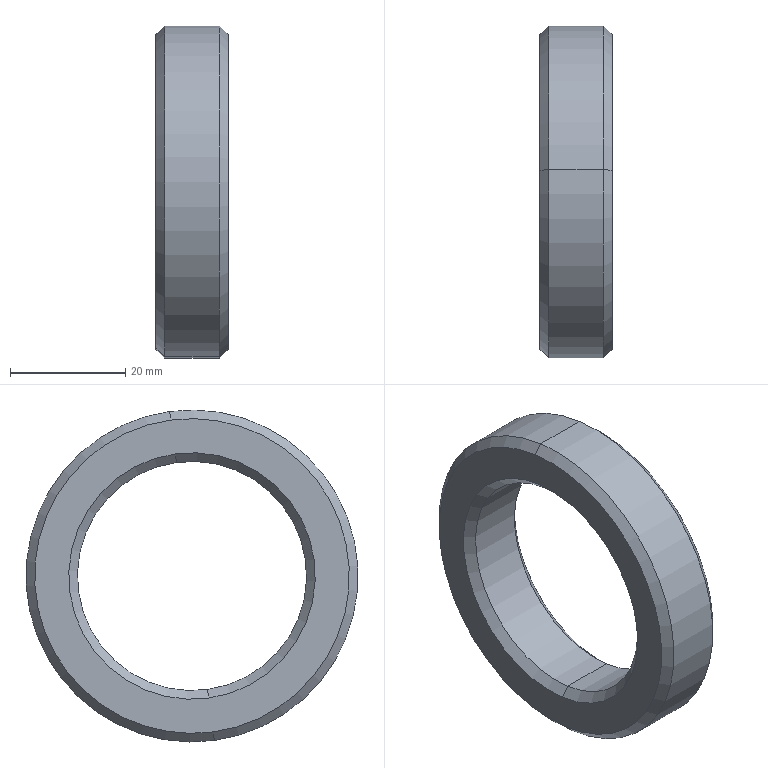Part | NX | features BREP 1 | 1 solid | 14 faces | box 12.5 x 57.5 x 57.5 mm | volume 16308 mm3 | cone 8 | cylinder 4 | plane 2 | commonest cylinder face diameters 39.688 x2 57.5 x2
STEP:
#1=CARTESIAN_POINT('',(-576.92,3.677,27.001));
#2=VERTEX_POINT('',#1);
#3=CARTESIAN_POINT('',(-576.92,-3.677,-27.001));
#4=VERTEX_POINT('',#3);
#5=CARTESIAN_POINT('',(-576.92,0.,0.));
#6=DIRECTION('',(-1.,0.,0.));
#7=DIRECTION('',(0.,0.1349,0.9909));
#8=AXIS2_PLACEMENT_3D('',#5,#6,#7);
#9=CIRCLE('',#8,27.25);
#10=EDGE_CURVE('',#2,#4,#9,.T.);
#11=ORIENTED_EDGE('',*,*,#10,.T.);
#12=CARTESIAN_POINT('',(-578.42,-3.879,-28.487));
#13=VERTEX_POINT('',#12);
#14=CARTESIAN_POINT('',(-576.92,-3.677,-27.001));
#15=DIRECTION('',(-0.7071,-0.09541,-0.7006));
#16=VECTOR('',#15,1000.);
#17=LINE('',#14,#16);
#18=EDGE_CURVE('',#4,#13,#17,.T.);
#19=ORIENTED_EDGE('',*,*,#18,.T.);
#20=CARTESIAN_POINT('',(-578.42,3.879,28.487));
#21=VERTEX_POINT('',#20);
#22=CARTESIAN_POINT('',(-578.42,0.,0.));
#23=DIRECTION('',(-1.,0.,0.));
#24=DIRECTION('',(0.,0.1349,0.9909));
#25=AXIS2_PLACEMENT_3D('',#22,#23,#24);
#26=CIRCLE('',#25,28.75);
#27=EDGE_CURVE('',#21,#13,#26,.T.);
#28=ORIENTED_EDGE('',*,*,#27,.F.);
#29=CARTESIAN_POINT('',(-576.92,3.677,27.001));
#30=DIRECTION('',(-0.7071,0.09541,0.7006));
#31=VECTOR('',#30,1000.);
#32=LINE('',#29,#31);
#33=EDGE_CURVE('',#2,#21,#32,.T.);
#34=ORIENTED_EDGE('',*,*,#33,.F.);
#35=EDGE_LOOP('',(#11,#19,#28,#34));
#36=FACE_BOUND('',#35,.T.);
#37=CARTESIAN_POINT('',(-576.92,0.,0.));
#38=DIRECTION('',(-1.,0.,0.));
#39=DIRECTION('',(0.,-0.1349,-0.9909));
#40=AXIS2_PLACEMENT_3D('',#37,#38,#39);
#41=CONICAL_SURFACE('',#40,27.25,0.7854);
#42=ADVANCED_FACE('',(#36),#41,.T.);
#43=CARTESIAN_POINT('',(-578.42,-2.678,-19.663));
#44=VERTEX_POINT('',#43);
#45=CARTESIAN_POINT('',(-578.42,2.678,19.663));
#46=VERTEX_POINT('',#45);
#47=CARTESIAN_POINT('',(-578.42,0.,0.));
#48=DIRECTION('',(-1.,0.,0.));
#49=DIRECTION('',(0.,0.1349,0.9909));
#50=AXIS2_PLACEMENT_3D('',#47,#48,#49);
#51=CIRCLE('',#50,19.844);
#52=EDGE_CURVE('',#44,#46,#51,.T.);
#53=ORIENTED_EDGE('',*,*,#52,.T.);
#54=CARTESIAN_POINT('',(-576.92,2.88,21.149));
#55=VERTEX_POINT('',#54);
#56=CARTESIAN_POINT('',(-578.42,2.678,19.663));
#57=DIRECTION('',(0.7071,0.09541,0.7006));
#58=VECTOR('',#57,1000.);
#59=LINE('',#56,#58);
#60=EDGE_CURVE('',#55,#46,#59,.F.);
#61=ORIENTED_EDGE('',*,*,#60,.F.);
#62=CARTESIAN_POINT('',(-576.92,-2.88,-21.149));
#63=VERTEX_POINT('',#62);
#64=CARTESIAN_POINT('',(-576.92,0.,0.));
#65=DIRECTION('',(-1.,0.,0.));
#66=DIRECTION('',(0.,0.1349,0.9909));
#67=AXIS2_PLACEMENT_3D('',#64,#65,#66);
#68=CIRCLE('',#67,21.344);
#69=EDGE_CURVE('',#63,#55,#68,.T.);
#70=ORIENTED_EDGE('',*,*,#69,.F.);
#71=CARTESIAN_POINT('',(-578.42,-2.678,-19.663));
#72=DIRECTION('',(0.7071,-0.09541,-0.7006));
#73=VECTOR('',#72,1000.);
#74=LINE('',#71,#73);
#75=EDGE_CURVE('',#63,#44,#74,.F.);
#76=ORIENTED_EDGE('',*,*,#75,.T.);
#77=EDGE_LOOP('',(#53,#61,#70,#76));
#78=FACE_BOUND('',#77,.T.);
#79=CARTESIAN_POINT('',(-578.42,0.,0.));
#80=DIRECTION('',(1.,0.,0.));
#81=DIRECTION('',(0.,0.1349,0.9909));
#82=AXIS2_PLACEMENT_3D('',#79,#80,#81);
#83=CONICAL_SURFACE('',#82,19.844,0.7854);
#84=ADVANCED_FACE('',(#78),#83,.F.);
#85=ORIENTED_EDGE('',*,*,#52,.F.);
#86=CARTESIAN_POINT('',(-587.92,-2.678,-19.663));
#87=VERTEX_POINT('',#86);
#88=CARTESIAN_POINT('',(-589.42,-2.678,-19.663));
#89=DIRECTION('',(-1.,0.,0.));
#90=VECTOR('',#89,1000.);
#91=LINE('',#88,#90);
#92=EDGE_CURVE('',#44,#87,#91,.T.);
#93=ORIENTED_EDGE('',*,*,#92,.T.);
#94=CARTESIAN_POINT('',(-587.92,2.678,19.663));
#95=VERTEX_POINT('',#94);
#96=CARTESIAN_POINT('',(-587.92,0.,0.));
#97=DIRECTION('',(-1.,0.,0.));
#98=DIRECTION('',(0.,0.1349,0.9909));
#99=AXIS2_PLACEMENT_3D('',#96,#97,#98);
#100=CIRCLE('',#99,19.844);
#101=EDGE_CURVE('',#87,#95,#100,.T.);
#102=ORIENTED_EDGE('',*,*,#101,.T.);
#103=CARTESIAN_POINT('',(-589.42,2.678,19.663));
#104=DIRECTION('',(-1.,0.,0.));
#105=VECTOR('',#104,1000.);
#106=LINE('',#103,#105);
#107=EDGE_CURVE('',#46,#95,#106,.T.);
#108=ORIENTED_EDGE('',*,*,#107,.F.);
#109=EDGE_LOOP('',(#85,#93,#102,#108));
#110=FACE_BOUND('',#109,.T.);
#111=CARTESIAN_POINT('',(-589.42,0.,0.));
#112=DIRECTION('',(-1.,0.,0.));
#113=DIRECTION('',(0.,-0.1349,-0.9909));
#114=AXIS2_PLACEMENT_3D('',#111,#112,#113);
#115=CYLINDRICAL_SURFACE('',#114,19.844);
#116=ADVANCED_FACE('',(#110),#115,.F.);
#117=ORIENTED_EDGE('',*,*,#101,.F.);
#118=CARTESIAN_POINT('',(-589.42,-2.88,-21.149));
#119=VERTEX_POINT('',#118);
#120=CARTESIAN_POINT('',(-589.42,-2.88,-21.149));
#121=DIRECTION('',(-0.7071,-0.09541,-0.7006));
#122=VECTOR('',#121,1000.);
#123=LINE('',#120,#122);
#124=EDGE_CURVE('',#87,#119,#123,.T.);
#125=ORIENTED_EDGE('',*,*,#124,.T.);
#126=CARTESIAN_POINT('',(-589.42,2.88,21.149));
#127=VERTEX_POINT('',#126);
#128=CARTESIAN_POINT('',(-589.42,0.,0.));
#129=DIRECTION('',(-1.,0.,0.));
#130=DIRECTION('',(0.,0.1349,0.9909));
#131=AXIS2_PLACEMENT_3D('',#128,#129,#130);
#132=CIRCLE('',#131,21.344);
#133=EDGE_CURVE('',#119,#127,#132,.T.);
#134=ORIENTED_EDGE('',*,*,#133,.T.);
#135=CARTESIAN_POINT('',(-589.42,2.88,21.149));
#136=DIRECTION('',(-0.7071,0.09541,0.7006));
#137=VECTOR('',#136,1000.);
#138=LINE('',#135,#137);
#139=EDGE_CURVE('',#95,#127,#138,.T.);
#140=ORIENTED_EDGE('',*,*,#139,.F.);
#141=EDGE_LOOP('',(#117,#125,#134,#140));
#142=FACE_BOUND('',#141,.T.);
#143=CARTESIAN_POINT('',(-589.42,0.,0.));
#144=DIRECTION('',(-1.,0.,0.));
#145=DIRECTION('',(0.,-0.1349,-0.9909));
#146=AXIS2_PLACEMENT_3D('',#143,#144,#145);
#147=CONICAL_SURFACE('',#146,21.344,0.7854);
#148=ADVANCED_FACE('',(#142),#147,.F.);
#149=CARTESIAN_POINT('',(-589.42,3.677,27.001));
#150=VERTEX_POINT('',#149);
#151=CARTESIAN_POINT('',(-589.42,-3.677,-27.001));
#152=VERTEX_POINT('',#151);
#153=CARTESIAN_POINT('',(-589.42,0.,0.));
#154=DIRECTION('',(-1.,0.,0.));
#155=DIRECTION('',(0.,0.1349,0.9909));
#156=AXIS2_PLACEMENT_3D('',#153,#154,#155);
#157=CIRCLE('',#156,27.25);
#158=EDGE_CURVE('',#150,#152,#157,.T.);
#159=ORIENTED_EDGE('',*,*,#158,.F.);
#160=CARTESIAN_POINT('',(-587.92,3.879,28.487));
#161=VERTEX_POINT('',#160);
#162=CARTESIAN_POINT('',(-587.92,3.879,28.487));
#163=DIRECTION('',(0.7071,0.09541,0.7006));
#164=VECTOR('',#163,1000.);
#165=LINE('',#162,#164);
#166=EDGE_CURVE('',#161,#150,#165,.F.);
#167=ORIENTED_EDGE('',*,*,#166,.F.);
#168=CARTESIAN_POINT('',(-587.92,-3.879,-28.487));
#169=VERTEX_POINT('',#168);
#170=CARTESIAN_POINT('',(-587.92,0.,0.));
#171=DIRECTION('',(-1.,0.,0.));
#172=DIRECTION('',(0.,0.1349,0.9909));
#173=AXIS2_PLACEMENT_3D('',#170,#171,#172);
#174=CIRCLE('',#173,28.75);
#175=EDGE_CURVE('',#161,#169,#174,.T.);
#176=ORIENTED_EDGE('',*,*,#175,.T.);
#177=CARTESIAN_POINT('',(-587.92,-3.879,-28.487));
#178=DIRECTION('',(0.7071,-0.09541,-0.7006));
#179=VECTOR('',#178,1000.);
#180=LINE('',#177,#179);
#181=EDGE_CURVE('',#169,#152,#180,.F.);
#182=ORIENTED_EDGE('',*,*,#181,.T.);
#183=EDGE_LOOP('',(#159,#167,#176,#182));
#184=FACE_BOUND('',#183,.T.);
#185=CARTESIAN_POINT('',(-587.92,0.,0.));
#186=DIRECTION('',(1.,0.,0.));
#187=DIRECTION('',(0.,0.1349,0.9909));
#188=AXIS2_PLACEMENT_3D('',#185,#186,#187);
#189=CONICAL_SURFACE('',#188,28.75,0.7854);
#190=ADVANCED_FACE('',(#184),#189,.T.);
#191=ORIENTED_EDGE('',*,*,#27,.T.);
#192=CARTESIAN_POINT('',(-589.42,-3.879,-28.487));
#193=DIRECTION('',(-1.,0.,0.));
#194=VECTOR('',#193,1000.);
#195=LINE('',#192,#194);
#196=EDGE_CURVE('',#13,#169,#195,.T.);
#197=ORIENTED_EDGE('',*,*,#196,.T.);
#198=ORIENTED_EDGE('',*,*,#175,.F.);
#199=CARTESIAN_POINT('',(-589.42,3.879,28.487));
#200=DIRECTION('',(-1.,0.,0.));
#201=VECTOR('',#200,1000.);
#202=LINE('',#199,#201);
#203=EDGE_CURVE('',#21,#161,#202,.T.);
#204=ORIENTED_EDGE('',*,*,#203,.F.);
#205=EDGE_LOOP('',(#191,#197,#198,#204));
#206=FACE_BOUND('',#205,.T.);
#207=CARTESIAN_POINT('',(-589.42,0.,0.));
#208=DIRECTION('',(-1.,0.,0.));
#209=DIRECTION('',(0.,-0.1349,-0.9909));
#210=AXIS2_PLACEMENT_3D('',#207,#208,#209);
#211=CYLINDRICAL_SURFACE('',#210,28.75);
#212=ADVANCED_FACE('',(#206),#211,.T.);
#213=ORIENTED_EDGE('',*,*,#196,.F.);
#214=CARTESIAN_POINT('',(-578.42,0.,0.));
#215=DIRECTION('',(-1.,0.,0.));
#216=DIRECTION('',(0.,0.1349,0.9909));
#217=AXIS2_PLACEMENT_3D('',#214,#215,#216);
#218=CIRCLE('',#217,28.75);
#219=EDGE_CURVE('',#13,#21,#218,.T.);
#220=ORIENTED_EDGE('',*,*,#219,.T.);
#221=ORIENTED_EDGE('',*,*,#203,.T.);
#222=CARTESIAN_POINT('',(-587.92,0.,0.));
#223=DIRECTION('',(-1.,0.,0.));
#224=DIRECTION('',(0.,0.1349,0.9909));
#225=AXIS2_PLACEMENT_3D('',#222,#223,#224);
#226=CIRCLE('',#225,28.75);
#227=EDGE_CURVE('',#169,#161,#226,.T.);
#228=ORIENTED_EDGE('',*,*,#227,.F.);
#229=EDGE_LOOP('',(#213,#220,#221,#228));
#230=FACE_BOUND('',#229,.T.);
#231=CARTESIAN_POINT('',(-589.42,0.,0.));
#232=DIRECTION('',(-1.,0.,0.));
#233=DIRECTION('',(0.,-0.1349,-0.9909));
#234=AXIS2_PLACEMENT_3D('',#231,#232,#233);
#235=CYLINDRICAL_SURFACE('',#234,28.75);
#236=ADVANCED_FACE('',(#230),#235,.T.);
#237=ORIENTED_EDGE('',*,*,#166,.T.);
#238=CARTESIAN_POINT('',(-589.42,0.,0.));
#239=DIRECTION('',(-1.,0.,0.));
#240=DIRECTION('',(0.,0.1349,0.9909));
#241=AXIS2_PLACEMENT_3D('',#238,#239,#240);
#242=CIRCLE('',#241,27.25);
#243=EDGE_CURVE('',#152,#150,#242,.T.);
#244=ORIENTED_EDGE('',*,*,#243,.F.);
#245=ORIENTED_EDGE('',*,*,#181,.F.);
#246=ORIENTED_EDGE('',*,*,#227,.T.);
#247=EDGE_LOOP('',(#237,#244,#245,#246));
#248=FACE_BOUND('',#247,.T.);
#249=CARTESIAN_POINT('',(-587.92,0.,0.));
#250=DIRECTION('',(1.,0.,0.));
#251=DIRECTION('',(0.,0.1349,0.9909));
#252=AXIS2_PLACEMENT_3D('',#249,#250,#251);
#253=CONICAL_SURFACE('',#252,28.75,0.7854);
#254=ADVANCED_FACE('',(#248),#253,.T.);
#255=CARTESIAN_POINT('',(-589.42,0.,0.));
#256=DIRECTION('',(-1.,0.,0.));
#257=DIRECTION('',(0.,0.1349,0.9909));
#258=AXIS2_PLACEMENT_3D('',#255,#256,#257);
#259=CIRCLE('',#258,21.344);
#260=EDGE_CURVE('',#127,#119,#259,.T.);
#261=ORIENTED_EDGE('',*,*,#260,.F.);
#262=ORIENTED_EDGE('',*,*,#133,.F.);
#263=EDGE_LOOP('',(#261,#262));
#264=FACE_BOUND('',#263,.T.);
#265=ORIENTED_EDGE('',*,*,#243,.T.);
#266=ORIENTED_EDGE('',*,*,#158,.T.);
#267=EDGE_LOOP('',(#265,#266));
#268=FACE_BOUND('',#267,.T.);
#269=CARTESIAN_POINT('',(-589.42,27.001,-3.677));
#270=DIRECTION('',(1.,0.,0.));
#271=DIRECTION('',(0.,0.1349,0.9909));
#272=AXIS2_PLACEMENT_3D('',#269,#270,#271);
#273=PLANE('',#272);
#274=ADVANCED_FACE('',(#264,#268),#273,.F.);
#275=ORIENTED_EDGE('',*,*,#124,.F.);
#276=CARTESIAN_POINT('',(-587.92,0.,0.));
#277=DIRECTION('',(-1.,0.,0.));
#278=DIRECTION('',(0.,0.1349,0.9909));
#279=AXIS2_PLACEMENT_3D('',#276,#277,#278);
#280=CIRCLE('',#279,19.844);
#281=EDGE_CURVE('',#95,#87,#280,.T.);
#282=ORIENTED_EDGE('',*,*,#281,.F.);
#283=ORIENTED_EDGE('',*,*,#139,.T.);
#284=ORIENTED_EDGE('',*,*,#260,.T.);
#285=EDGE_LOOP('',(#275,#282,#283,#284));
#286=FACE_BOUND('',#285,.T.);
#287=CARTESIAN_POINT('',(-589.42,0.,0.));
#288=DIRECTION('',(-1.,0.,0.));
#289=DIRECTION('',(0.,-0.1349,-0.9909));
#290=AXIS2_PLACEMENT_3D('',#287,#288,#289);
#291=CONICAL_SURFACE('',#290,21.344,0.7854);
#292=ADVANCED_FACE('',(#286),#291,.F.);
#293=ORIENTED_EDGE('',*,*,#92,.F.);
#294=CARTESIAN_POINT('',(-578.42,0.,0.));
#295=DIRECTION('',(-1.,0.,0.));
#296=DIRECTION('',(0.,0.1349,0.9909));
#297=AXIS2_PLACEMENT_3D('',#294,#295,#296);
#298=CIRCLE('',#297,19.844);
#299=EDGE_CURVE('',#46,#44,#298,.T.);
#300=ORIENTED_EDGE('',*,*,#299,.F.);
#301=ORIENTED_EDGE('',*,*,#107,.T.);
#302=ORIENTED_EDGE('',*,*,#281,.T.);
#303=EDGE_LOOP('',(#293,#300,#301,#302));
#304=FACE_BOUND('',#303,.T.);
#305=CARTESIAN_POINT('',(-589.42,0.,0.));
#306=DIRECTION('',(-1.,0.,0.));
#307=DIRECTION('',(0.,-0.1349,-0.9909));
#308=AXIS2_PLACEMENT_3D('',#305,#306,#307);
#309=CYLINDRICAL_SURFACE('',#308,19.844);
#310=ADVANCED_FACE('',(#304),#309,.F.);
#311=ORIENTED_EDGE('',*,*,#60,.T.);
#312=ORIENTED_EDGE('',*,*,#299,.T.);
#313=ORIENTED_EDGE('',*,*,#75,.F.);
#314=CARTESIAN_POINT('',(-576.92,0.,0.));
#315=DIRECTION('',(-1.,0.,0.));
#316=DIRECTION('',(0.,0.1349,0.9909));
#317=AXIS2_PLACEMENT_3D('',#314,#315,#316);
#318=CIRCLE('',#317,21.344);
#319=EDGE_CURVE('',#55,#63,#318,.T.);
#320=ORIENTED_EDGE('',*,*,#319,.F.);
#321=EDGE_LOOP('',(#311,#312,#313,#320));
#322=FACE_BOUND('',#321,.T.);
#323=CARTESIAN_POINT('',(-578.42,0.,0.));
#324=DIRECTION('',(1.,0.,0.));
#325=DIRECTION('',(0.,0.1349,0.9909));
#326=AXIS2_PLACEMENT_3D('',#323,#324,#325);
#327=CONICAL_SURFACE('',#326,19.844,0.7854);
#328=ADVANCED_FACE('',(#322),#327,.F.);
#329=ORIENTED_EDGE('',*,*,#10,.F.);
#330=CARTESIAN_POINT('',(-576.92,0.,0.));
#331=DIRECTION('',(-1.,0.,0.));
#332=DIRECTION('',(0.,0.1349,0.9909));
#333=AXIS2_PLACEMENT_3D('',#330,#331,#332);
#334=CIRCLE('',#333,27.25);
#335=EDGE_CURVE('',#4,#2,#334,.T.);
#336=ORIENTED_EDGE('',*,*,#335,.F.);
#337=EDGE_LOOP('',(#329,#336));
#338=FACE_BOUND('',#337,.T.);
#339=ORIENTED_EDGE('',*,*,#69,.T.);
#340=ORIENTED_EDGE('',*,*,#319,.T.);
#341=EDGE_LOOP('',(#339,#340));
#342=FACE_BOUND('',#341,.T.);
#343=CARTESIAN_POINT('',(-576.92,21.149,-2.88));
#344=DIRECTION('',(-1.,0.,0.));
#345=DIRECTION('',(0.,-0.1349,-0.9909));
#346=AXIS2_PLACEMENT_3D('',#343,#344,#345);
#347=PLANE('',#346);
#348=ADVANCED_FACE('',(#338,#342),#347,.F.);
#349=ORIENTED_EDGE('',*,*,#18,.F.);
#350=ORIENTED_EDGE('',*,*,#335,.T.);
#351=ORIENTED_EDGE('',*,*,#33,.T.);
#352=ORIENTED_EDGE('',*,*,#219,.F.);
#353=EDGE_LOOP('',(#349,#350,#351,#352));
#354=FACE_BOUND('',#353,.T.);
#355=CARTESIAN_POINT('',(-576.92,0.,0.));
#356=DIRECTION('',(-1.,0.,0.));
#357=DIRECTION('',(0.,-0.1349,-0.9909));
#358=AXIS2_PLACEMENT_3D('',#355,#356,#357);
#359=CONICAL_SURFACE('',#358,27.25,0.7854);
#360=ADVANCED_FACE('',(#354),#359,.T.);
#361=CLOSED_SHELL('',(#42,#84,#116,#148,#190,#212,#236,#254,#274,#292,#310,#328,#348,#360));
#362=MANIFOLD_SOLID_BREP('',#361);
#363=(LENGTH_UNIT()NAMED_UNIT(*)SI_UNIT(.MILLI.,.METRE.));
#364=UNCERTAINTY_MEASURE_WITH_UNIT(LENGTH_MEASURE(0.00001),#363,'','');
#365=(NAMED_UNIT(*)PLANE_ANGLE_UNIT()SI_UNIT($,.RADIAN.));
#366=(NAMED_UNIT(*)SI_UNIT($,.STERADIAN.)SOLID_ANGLE_UNIT());
#367=(GEOMETRIC_REPRESENTATION_CONTEXT(3)GLOBAL_UNCERTAINTY_ASSIGNED_CONTEXT((#364))GLOBAL_UNIT_ASSIGNED_CONTEXT((#363,#365,#366))REPRESENTATION_CONTEXT('',''));
#368=ADVANCED_BREP_SHAPE_REPRESENTATION('',(#362),#367);